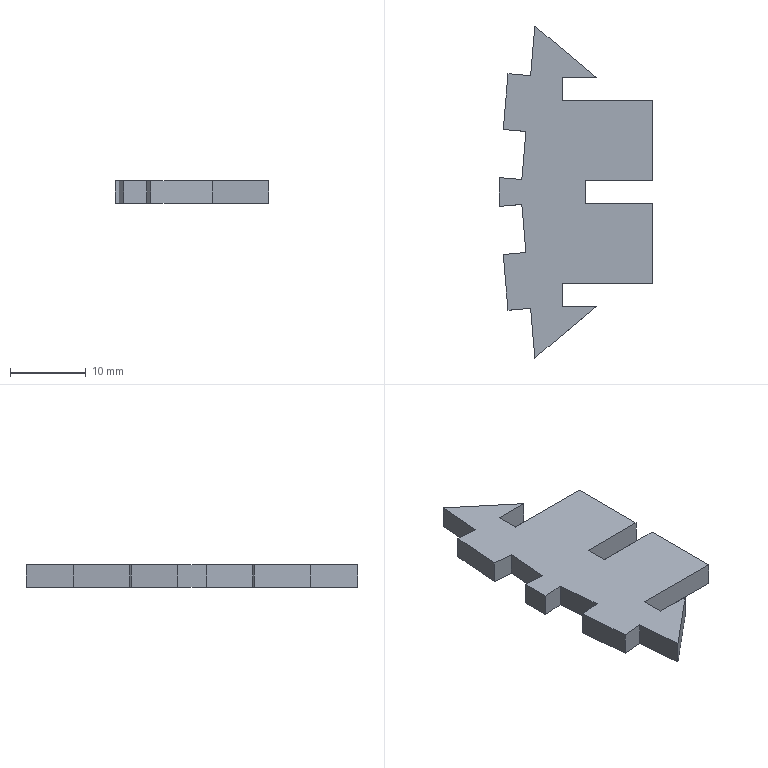Part | SolidWorks | features BaseBody 1 | 1 solid | 28 faces | box 20.269 x 43.799 x 3 mm | volume 1567 mm3 | plane 28
STEP:
#1=CARTESIAN_POINT('',(-11.851,-12.08,-1.5));
#2=VERTEX_POINT('',#1);
#3=CARTESIAN_POINT('',(0.1003,-12.082,-1.5));
#4=VERTEX_POINT('',#3);
#5=CARTESIAN_POINT('',(-0.002246,-12.082,-1.5));
#6=DIRECTION('',(1.,-0.0001859,0.));
#7=VECTOR('',#6,1000.);
#8=LINE('',#5,#7);
#9=EDGE_CURVE('',#2,#4,#8,.T.);
#10=ORIENTED_EDGE('',*,*,#9,.F.);
#11=CARTESIAN_POINT('',(-11.851,-15.077,-1.5));
#12=VERTEX_POINT('',#11);
#13=CARTESIAN_POINT('',(-11.851,0.,-1.5));
#14=DIRECTION('',(0.,1.,0.));
#15=VECTOR('',#14,1000.);
#16=LINE('',#13,#15);
#17=EDGE_CURVE('',#12,#2,#16,.T.);
#18=ORIENTED_EDGE('',*,*,#17,.F.);
#19=CARTESIAN_POINT('',(-7.293,-15.074,-1.5));
#20=VERTEX_POINT('',#19);
#21=CARTESIAN_POINT('',(0.009187,-15.07,-1.5));
#22=DIRECTION('',(-1.,-0.0006096,0.));
#23=VECTOR('',#22,1000.);
#24=LINE('',#21,#23);
#25=EDGE_CURVE('',#20,#12,#24,.T.);
#26=ORIENTED_EDGE('',*,*,#25,.F.);
#27=CARTESIAN_POINT('',(-15.47,-21.897,-1.5));
#28=VERTEX_POINT('',#27);
#29=CARTESIAN_POINT('',(4.421,-5.299,-1.5));
#30=DIRECTION('',(0.7678,0.6407,0.));
#31=VECTOR('',#30,1000.);
#32=LINE('',#29,#31);
#33=EDGE_CURVE('',#28,#20,#32,.T.);
#34=ORIENTED_EDGE('',*,*,#33,.F.);
#35=CARTESIAN_POINT('',(-16.025,-15.349,-1.5));
#36=VERTEX_POINT('',#35);
#37=CARTESIAN_POINT('',(-17.203,-1.458,-1.5));
#38=DIRECTION('',(0.08445,-0.9964,0.));
#39=VECTOR('',#38,1000.);
#40=LINE('',#37,#39);
#41=EDGE_CURVE('',#36,#28,#40,.T.);
#42=ORIENTED_EDGE('',*,*,#41,.F.);
#43=CARTESIAN_POINT('',(-19.01,-15.602,-1.5));
#44=VERTEX_POINT('',#43);
#45=CARTESIAN_POINT('',(1.175,-13.895,-1.5));
#46=DIRECTION('',(0.9964,0.08424,0.));
#47=VECTOR('',#46,1000.);
#48=LINE('',#45,#47);
#49=EDGE_CURVE('',#44,#36,#48,.T.);
#50=ORIENTED_EDGE('',*,*,#49,.F.);
#51=CARTESIAN_POINT('',(-19.632,-8.242,-1.5));
#52=VERTEX_POINT('',#51);
#53=CARTESIAN_POINT('',(-20.184,-1.706,-1.5));
#54=DIRECTION('',(0.08424,-0.9964,0.));
#55=VECTOR('',#54,1000.);
#56=LINE('',#53,#55);
#57=EDGE_CURVE('',#52,#44,#56,.T.);
#58=ORIENTED_EDGE('',*,*,#57,.F.);
#59=CARTESIAN_POINT('',(-16.646,-7.989,-1.5));
#60=VERTEX_POINT('',#59);
#61=CARTESIAN_POINT('',(0.5525,-6.535,-1.5));
#62=DIRECTION('',(-0.9964,-0.08424,0.));
#63=VECTOR('',#62,1000.);
#64=LINE('',#61,#63);
#65=EDGE_CURVE('',#60,#52,#64,.T.);
#66=ORIENTED_EDGE('',*,*,#65,.F.);
#67=CARTESIAN_POINT('',(-17.182,-1.643,-1.5));
#68=VERTEX_POINT('',#67);
#69=CARTESIAN_POINT('',(-17.198,-1.453,-1.5));
#70=DIRECTION('',(0.08416,-0.9965,0.));
#71=VECTOR('',#70,1000.);
#72=LINE('',#69,#71);
#73=EDGE_CURVE('',#68,#60,#72,.T.);
#74=ORIENTED_EDGE('',*,*,#73,.F.);
#75=CARTESIAN_POINT('',(-20.169,-1.897,-1.5));
#76=VERTEX_POINT('',#75);
#77=CARTESIAN_POINT('',(0.01566,-0.1847,-1.5));
#78=DIRECTION('',(0.9964,0.08451,0.));
#79=VECTOR('',#78,1000.);
#80=LINE('',#77,#79);
#81=EDGE_CURVE('',#76,#68,#80,.T.);
#82=ORIENTED_EDGE('',*,*,#81,.F.);
#83=CARTESIAN_POINT('',(-20.169,1.901,-1.5));
#84=VERTEX_POINT('',#83);
#85=CARTESIAN_POINT('',(-20.169,0.,-1.5));
#86=DIRECTION('',(0.,-1.,0.));
#87=VECTOR('',#86,1000.);
#88=LINE('',#85,#87);
#89=EDGE_CURVE('',#84,#76,#88,.T.);
#90=ORIENTED_EDGE('',*,*,#89,.F.);
#91=CARTESIAN_POINT('',(-17.182,1.648,-1.5));
#92=VERTEX_POINT('',#91);
#93=CARTESIAN_POINT('',(0.01606,0.1893,-1.5));
#94=DIRECTION('',(-0.9964,0.08451,0.));
#95=VECTOR('',#94,1000.);
#96=LINE('',#93,#95);
#97=EDGE_CURVE('',#92,#84,#96,.T.);
#98=ORIENTED_EDGE('',*,*,#97,.F.);
#99=CARTESIAN_POINT('',(-16.646,7.994,-1.5));
#100=VERTEX_POINT('',#99);
#101=CARTESIAN_POINT('',(-17.199,1.453,-1.5));
#102=DIRECTION('',(-0.08416,-0.9965,0.));
#103=VECTOR('',#102,1000.);
#104=LINE('',#101,#103);
#105=EDGE_CURVE('',#100,#92,#104,.T.);
#106=ORIENTED_EDGE('',*,*,#105,.F.);
#107=CARTESIAN_POINT('',(-19.632,8.246,-1.5));
#108=VERTEX_POINT('',#107);
#109=CARTESIAN_POINT('',(0.5529,6.54,-1.5));
#110=DIRECTION('',(0.9964,-0.08424,0.));
#111=VECTOR('',#110,1000.);
#112=LINE('',#109,#111);
#113=EDGE_CURVE('',#108,#100,#112,.T.);
#114=ORIENTED_EDGE('',*,*,#113,.F.);
#115=CARTESIAN_POINT('',(-19.01,15.606,-1.5));
#116=VERTEX_POINT('',#115);
#117=CARTESIAN_POINT('',(-20.185,1.706,-1.5));
#118=DIRECTION('',(-0.08424,-0.9964,0.));
#119=VECTOR('',#118,1000.);
#120=LINE('',#117,#119);
#121=EDGE_CURVE('',#116,#108,#120,.T.);
#122=ORIENTED_EDGE('',*,*,#121,.F.);
#123=CARTESIAN_POINT('',(-16.025,15.354,-1.5));
#124=VERTEX_POINT('',#123);
#125=CARTESIAN_POINT('',(1.175,13.9,-1.5));
#126=DIRECTION('',(-0.9964,0.08424,0.));
#127=VECTOR('',#126,1000.);
#128=LINE('',#125,#127);
#129=EDGE_CURVE('',#124,#116,#128,.T.);
#130=ORIENTED_EDGE('',*,*,#129,.F.);
#131=CARTESIAN_POINT('',(-15.47,21.902,-1.5));
#132=VERTEX_POINT('',#131);
#133=CARTESIAN_POINT('',(-17.203,1.458,-1.5));
#134=DIRECTION('',(-0.08445,-0.9964,0.));
#135=VECTOR('',#134,1000.);
#136=LINE('',#133,#135);
#137=EDGE_CURVE('',#132,#124,#136,.T.);
#138=ORIENTED_EDGE('',*,*,#137,.F.);
#139=CARTESIAN_POINT('',(-7.293,15.079,-1.5));
#140=VERTEX_POINT('',#139);
#141=CARTESIAN_POINT('',(4.424,5.301,-1.5));
#142=DIRECTION('',(-0.7678,0.6407,0.));
#143=VECTOR('',#142,1000.);
#144=LINE('',#141,#143);
#145=EDGE_CURVE('',#140,#132,#144,.T.);
#146=ORIENTED_EDGE('',*,*,#145,.F.);
#147=CARTESIAN_POINT('',(-11.851,15.082,-1.5));
#148=VERTEX_POINT('',#147);
#149=CARTESIAN_POINT('',(0.00919,15.074,-1.5));
#150=DIRECTION('',(1.,-0.0006096,0.));
#151=VECTOR('',#150,1000.);
#152=LINE('',#149,#151);
#153=EDGE_CURVE('',#148,#140,#152,.T.);
#154=ORIENTED_EDGE('',*,*,#153,.F.);
#155=CARTESIAN_POINT('',(-11.851,12.084,-1.5));
#156=VERTEX_POINT('',#155);
#157=CARTESIAN_POINT('',(-11.851,0.,-1.5));
#158=DIRECTION('',(0.,1.,0.));
#159=VECTOR('',#158,1000.);
#160=LINE('',#157,#159);
#161=EDGE_CURVE('',#156,#148,#160,.T.);
#162=ORIENTED_EDGE('',*,*,#161,.F.);
#163=CARTESIAN_POINT('',(0.1003,12.086,-1.5));
#164=VERTEX_POINT('',#163);
#165=CARTESIAN_POINT('',(-0.002247,12.086,-1.5));
#166=DIRECTION('',(-1.,-0.0001859,0.));
#167=VECTOR('',#166,1000.);
#168=LINE('',#165,#167);
#169=EDGE_CURVE('',#164,#156,#168,.T.);
#170=ORIENTED_EDGE('',*,*,#169,.F.);
#171=CARTESIAN_POINT('',(0.1003,1.498,-1.5));
#172=VERTEX_POINT('',#171);
#173=CARTESIAN_POINT('',(0.1003,0.,-1.5));
#174=DIRECTION('',(0.,1.,0.));
#175=VECTOR('',#174,1000.);
#176=LINE('',#173,#175);
#177=EDGE_CURVE('',#172,#164,#176,.T.);
#178=ORIENTED_EDGE('',*,*,#177,.F.);
#179=CARTESIAN_POINT('',(-8.819,1.498,-1.5));
#180=VERTEX_POINT('',#179);
#181=CARTESIAN_POINT('',(0.,1.498,-1.5));
#182=DIRECTION('',(1.,0.,0.));
#183=VECTOR('',#182,1000.);
#184=LINE('',#181,#183);
#185=EDGE_CURVE('',#180,#172,#184,.T.);
#186=ORIENTED_EDGE('',*,*,#185,.F.);
#187=CARTESIAN_POINT('',(-8.819,-1.498,-1.5));
#188=VERTEX_POINT('',#187);
#189=CARTESIAN_POINT('',(-8.819,0.,-1.5));
#190=DIRECTION('',(0.,1.,0.));
#191=VECTOR('',#190,1000.);
#192=LINE('',#189,#191);
#193=EDGE_CURVE('',#188,#180,#192,.T.);
#194=ORIENTED_EDGE('',*,*,#193,.F.);
#195=CARTESIAN_POINT('',(0.1003,-1.498,-1.5));
#196=VERTEX_POINT('',#195);
#197=CARTESIAN_POINT('',(0.,-1.498,-1.5));
#198=DIRECTION('',(-1.,0.,0.));
#199=VECTOR('',#198,1000.);
#200=LINE('',#197,#199);
#201=EDGE_CURVE('',#196,#188,#200,.T.);
#202=ORIENTED_EDGE('',*,*,#201,.F.);
#203=CARTESIAN_POINT('',(0.1003,0.,-1.5));
#204=DIRECTION('',(0.,1.,0.));
#205=VECTOR('',#204,1000.);
#206=LINE('',#203,#205);
#207=EDGE_CURVE('',#4,#196,#206,.T.);
#208=ORIENTED_EDGE('',*,*,#207,.F.);
#209=EDGE_LOOP('',(#10,#18,#26,#34,#42,#50,#58,#66,#74,#82,#90,#98,#106,#114,#122,#130,#138,#146,#154,#162,#170,#178,#186,#194,#202,#208));
#210=FACE_OUTER_BOUND('',#209,.T.);
#211=CARTESIAN_POINT('',(0.,0.,-1.5));
#212=DIRECTION('',(0.,0.,1.));
#213=DIRECTION('',(1.,0.,0.));
#214=AXIS2_PLACEMENT_3D('',#211,#212,#213);
#215=PLANE('',#214);
#216=ADVANCED_FACE('',(#210),#215,.F.);
#217=CARTESIAN_POINT('',(-11.851,-12.08,1.5));
#218=VERTEX_POINT('',#217);
#219=CARTESIAN_POINT('',(0.1003,-12.082,1.5));
#220=VERTEX_POINT('',#219);
#221=CARTESIAN_POINT('',(-0.002246,-12.082,1.5));
#222=DIRECTION('',(1.,-0.0001859,0.));
#223=VECTOR('',#222,1000.);
#224=LINE('',#221,#223);
#225=EDGE_CURVE('',#218,#220,#224,.T.);
#226=ORIENTED_EDGE('',*,*,#225,.T.);
#227=CARTESIAN_POINT('',(0.1003,-1.498,1.5));
#228=VERTEX_POINT('',#227);
#229=CARTESIAN_POINT('',(0.1003,0.,1.5));
#230=DIRECTION('',(0.,1.,0.));
#231=VECTOR('',#230,1000.);
#232=LINE('',#229,#231);
#233=EDGE_CURVE('',#220,#228,#232,.T.);
#234=ORIENTED_EDGE('',*,*,#233,.T.);
#235=CARTESIAN_POINT('',(-8.819,-1.498,1.5));
#236=VERTEX_POINT('',#235);
#237=CARTESIAN_POINT('',(0.,-1.498,1.5));
#238=DIRECTION('',(-1.,0.,0.));
#239=VECTOR('',#238,1000.);
#240=LINE('',#237,#239);
#241=EDGE_CURVE('',#228,#236,#240,.T.);
#242=ORIENTED_EDGE('',*,*,#241,.T.);
#243=CARTESIAN_POINT('',(-8.819,1.498,1.5));
#244=VERTEX_POINT('',#243);
#245=CARTESIAN_POINT('',(-8.819,0.,1.5));
#246=DIRECTION('',(0.,1.,0.));
#247=VECTOR('',#246,1000.);
#248=LINE('',#245,#247);
#249=EDGE_CURVE('',#236,#244,#248,.T.);
#250=ORIENTED_EDGE('',*,*,#249,.T.);
#251=CARTESIAN_POINT('',(0.1003,1.498,1.5));
#252=VERTEX_POINT('',#251);
#253=CARTESIAN_POINT('',(0.,1.498,1.5));
#254=DIRECTION('',(1.,0.,0.));
#255=VECTOR('',#254,1000.);
#256=LINE('',#253,#255);
#257=EDGE_CURVE('',#244,#252,#256,.T.);
#258=ORIENTED_EDGE('',*,*,#257,.T.);
#259=CARTESIAN_POINT('',(0.1003,12.086,1.5));
#260=VERTEX_POINT('',#259);
#261=CARTESIAN_POINT('',(0.1003,0.,1.5));
#262=DIRECTION('',(0.,1.,0.));
#263=VECTOR('',#262,1000.);
#264=LINE('',#261,#263);
#265=EDGE_CURVE('',#252,#260,#264,.T.);
#266=ORIENTED_EDGE('',*,*,#265,.T.);
#267=CARTESIAN_POINT('',(-11.851,12.084,1.5));
#268=VERTEX_POINT('',#267);
#269=CARTESIAN_POINT('',(-0.002247,12.086,1.5));
#270=DIRECTION('',(-1.,-0.0001859,0.));
#271=VECTOR('',#270,1000.);
#272=LINE('',#269,#271);
#273=EDGE_CURVE('',#260,#268,#272,.T.);
#274=ORIENTED_EDGE('',*,*,#273,.T.);
#275=CARTESIAN_POINT('',(-11.851,15.082,1.5));
#276=VERTEX_POINT('',#275);
#277=CARTESIAN_POINT('',(-11.851,0.,1.5));
#278=DIRECTION('',(0.,1.,0.));
#279=VECTOR('',#278,1000.);
#280=LINE('',#277,#279);
#281=EDGE_CURVE('',#268,#276,#280,.T.);
#282=ORIENTED_EDGE('',*,*,#281,.T.);
#283=CARTESIAN_POINT('',(-7.293,15.079,1.5));
#284=VERTEX_POINT('',#283);
#285=CARTESIAN_POINT('',(0.00919,15.074,1.5));
#286=DIRECTION('',(1.,-0.0006096,0.));
#287=VECTOR('',#286,1000.);
#288=LINE('',#285,#287);
#289=EDGE_CURVE('',#276,#284,#288,.T.);
#290=ORIENTED_EDGE('',*,*,#289,.T.);
#291=CARTESIAN_POINT('',(-15.47,21.902,1.5));
#292=VERTEX_POINT('',#291);
#293=CARTESIAN_POINT('',(4.424,5.301,1.5));
#294=DIRECTION('',(-0.7678,0.6407,0.));
#295=VECTOR('',#294,1000.);
#296=LINE('',#293,#295);
#297=EDGE_CURVE('',#284,#292,#296,.T.);
#298=ORIENTED_EDGE('',*,*,#297,.T.);
#299=CARTESIAN_POINT('',(-16.025,15.354,1.5));
#300=VERTEX_POINT('',#299);
#301=CARTESIAN_POINT('',(-17.203,1.458,1.5));
#302=DIRECTION('',(-0.08445,-0.9964,0.));
#303=VECTOR('',#302,1000.);
#304=LINE('',#301,#303);
#305=EDGE_CURVE('',#292,#300,#304,.T.);
#306=ORIENTED_EDGE('',*,*,#305,.T.);
#307=CARTESIAN_POINT('',(-19.01,15.606,1.5));
#308=VERTEX_POINT('',#307);
#309=CARTESIAN_POINT('',(1.175,13.9,1.5));
#310=DIRECTION('',(-0.9964,0.08424,0.));
#311=VECTOR('',#310,1000.);
#312=LINE('',#309,#311);
#313=EDGE_CURVE('',#300,#308,#312,.T.);
#314=ORIENTED_EDGE('',*,*,#313,.T.);
#315=CARTESIAN_POINT('',(-19.632,8.246,1.5));
#316=VERTEX_POINT('',#315);
#317=CARTESIAN_POINT('',(-20.185,1.706,1.5));
#318=DIRECTION('',(-0.08424,-0.9964,0.));
#319=VECTOR('',#318,1000.);
#320=LINE('',#317,#319);
#321=EDGE_CURVE('',#308,#316,#320,.T.);
#322=ORIENTED_EDGE('',*,*,#321,.T.);
#323=CARTESIAN_POINT('',(-16.646,7.994,1.5));
#324=VERTEX_POINT('',#323);
#325=CARTESIAN_POINT('',(0.5529,6.54,1.5));
#326=DIRECTION('',(0.9964,-0.08424,0.));
#327=VECTOR('',#326,1000.);
#328=LINE('',#325,#327);
#329=EDGE_CURVE('',#316,#324,#328,.T.);
#330=ORIENTED_EDGE('',*,*,#329,.T.);
#331=CARTESIAN_POINT('',(-17.182,1.648,1.5));
#332=VERTEX_POINT('',#331);
#333=CARTESIAN_POINT('',(-17.199,1.453,1.5));
#334=DIRECTION('',(-0.08416,-0.9965,0.));
#335=VECTOR('',#334,1000.);
#336=LINE('',#333,#335);
#337=EDGE_CURVE('',#324,#332,#336,.T.);
#338=ORIENTED_EDGE('',*,*,#337,.T.);
#339=CARTESIAN_POINT('',(-20.169,1.901,1.5));
#340=VERTEX_POINT('',#339);
#341=CARTESIAN_POINT('',(0.01606,0.1893,1.5));
#342=DIRECTION('',(-0.9964,0.08451,0.));
#343=VECTOR('',#342,1000.);
#344=LINE('',#341,#343);
#345=EDGE_CURVE('',#332,#340,#344,.T.);
#346=ORIENTED_EDGE('',*,*,#345,.T.);
#347=CARTESIAN_POINT('',(-20.169,-1.897,1.5));
#348=VERTEX_POINT('',#347);
#349=CARTESIAN_POINT('',(-20.169,0.,1.5));
#350=DIRECTION('',(0.,-1.,0.));
#351=VECTOR('',#350,1000.);
#352=LINE('',#349,#351);
#353=EDGE_CURVE('',#340,#348,#352,.T.);
#354=ORIENTED_EDGE('',*,*,#353,.T.);
#355=CARTESIAN_POINT('',(-17.182,-1.643,1.5));
#356=VERTEX_POINT('',#355);
#357=CARTESIAN_POINT('',(0.01566,-0.1847,1.5));
#358=DIRECTION('',(0.9964,0.08451,0.));
#359=VECTOR('',#358,1000.);
#360=LINE('',#357,#359);
#361=EDGE_CURVE('',#348,#356,#360,.T.);
#362=ORIENTED_EDGE('',*,*,#361,.T.);
#363=CARTESIAN_POINT('',(-16.646,-7.989,1.5));
#364=VERTEX_POINT('',#363);
#365=CARTESIAN_POINT('',(-17.198,-1.453,1.5));
#366=DIRECTION('',(0.08416,-0.9965,0.));
#367=VECTOR('',#366,1000.);
#368=LINE('',#365,#367);
#369=EDGE_CURVE('',#356,#364,#368,.T.);
#370=ORIENTED_EDGE('',*,*,#369,.T.);
#371=CARTESIAN_POINT('',(-19.632,-8.242,1.5));
#372=VERTEX_POINT('',#371);
#373=CARTESIAN_POINT('',(0.5525,-6.535,1.5));
#374=DIRECTION('',(-0.9964,-0.08424,0.));
#375=VECTOR('',#374,1000.);
#376=LINE('',#373,#375);
#377=EDGE_CURVE('',#364,#372,#376,.T.);
#378=ORIENTED_EDGE('',*,*,#377,.T.);
#379=CARTESIAN_POINT('',(-19.01,-15.602,1.5));
#380=VERTEX_POINT('',#379);
#381=CARTESIAN_POINT('',(-20.184,-1.706,1.5));
#382=DIRECTION('',(0.08424,-0.9964,0.));
#383=VECTOR('',#382,1000.);
#384=LINE('',#381,#383);
#385=EDGE_CURVE('',#372,#380,#384,.T.);
#386=ORIENTED_EDGE('',*,*,#385,.T.);
#387=CARTESIAN_POINT('',(-16.025,-15.349,1.5));
#388=VERTEX_POINT('',#387);
#389=CARTESIAN_POINT('',(1.175,-13.895,1.5));
#390=DIRECTION('',(0.9964,0.08424,0.));
#391=VECTOR('',#390,1000.);
#392=LINE('',#389,#391);
#393=EDGE_CURVE('',#380,#388,#392,.T.);
#394=ORIENTED_EDGE('',*,*,#393,.T.);
#395=CARTESIAN_POINT('',(-15.47,-21.897,1.5));
#396=VERTEX_POINT('',#395);
#397=CARTESIAN_POINT('',(-17.203,-1.458,1.5));
#398=DIRECTION('',(0.08445,-0.9964,0.));
#399=VECTOR('',#398,1000.);
#400=LINE('',#397,#399);
#401=EDGE_CURVE('',#388,#396,#400,.T.);
#402=ORIENTED_EDGE('',*,*,#401,.T.);
#403=CARTESIAN_POINT('',(-7.293,-15.074,1.5));
#404=VERTEX_POINT('',#403);
#405=CARTESIAN_POINT('',(4.421,-5.299,1.5));
#406=DIRECTION('',(0.7678,0.6407,0.));
#407=VECTOR('',#406,1000.);
#408=LINE('',#405,#407);
#409=EDGE_CURVE('',#396,#404,#408,.T.);
#410=ORIENTED_EDGE('',*,*,#409,.T.);
#411=CARTESIAN_POINT('',(-11.851,-15.077,1.5));
#412=VERTEX_POINT('',#411);
#413=CARTESIAN_POINT('',(0.009187,-15.07,1.5));
#414=DIRECTION('',(-1.,-0.0006096,0.));
#415=VECTOR('',#414,1000.);
#416=LINE('',#413,#415);
#417=EDGE_CURVE('',#404,#412,#416,.T.);
#418=ORIENTED_EDGE('',*,*,#417,.T.);
#419=CARTESIAN_POINT('',(-11.851,0.,1.5));
#420=DIRECTION('',(0.,1.,0.));
#421=VECTOR('',#420,1000.);
#422=LINE('',#419,#421);
#423=EDGE_CURVE('',#412,#218,#422,.T.);
#424=ORIENTED_EDGE('',*,*,#423,.T.);
#425=EDGE_LOOP('',(#226,#234,#242,#250,#258,#266,#274,#282,#290,#298,#306,#314,#322,#330,#338,#346,#354,#362,#370,#378,#386,#394,#402,#410,#418,#424));
#426=FACE_OUTER_BOUND('',#425,.T.);
#427=CARTESIAN_POINT('',(0.,0.,1.5));
#428=DIRECTION('',(0.,0.,1.));
#429=DIRECTION('',(1.,0.,0.));
#430=AXIS2_PLACEMENT_3D('',#427,#428,#429);
#431=PLANE('',#430);
#432=ADVANCED_FACE('',(#426),#431,.T.);
#433=ORIENTED_EDGE('',*,*,#17,.T.);
#434=CARTESIAN_POINT('',(-11.851,-12.08,1.5));
#435=DIRECTION('',(0.,0.,-1.));
#436=VECTOR('',#435,1000.);
#437=LINE('',#434,#436);
#438=EDGE_CURVE('',#218,#2,#437,.T.);
#439=ORIENTED_EDGE('',*,*,#438,.F.);
#440=ORIENTED_EDGE('',*,*,#423,.F.);
#441=CARTESIAN_POINT('',(-11.851,-15.077,1.5));
#442=DIRECTION('',(0.,0.,-1.));
#443=VECTOR('',#442,1000.);
#444=LINE('',#441,#443);
#445=EDGE_CURVE('',#412,#12,#444,.T.);
#446=ORIENTED_EDGE('',*,*,#445,.T.);
#447=EDGE_LOOP('',(#433,#439,#440,#446));
#448=FACE_OUTER_BOUND('',#447,.T.);
#449=CARTESIAN_POINT('',(-11.851,0.,1.5));
#450=DIRECTION('',(-1.,0.,0.));
#451=DIRECTION('',(0.,0.,1.));
#452=AXIS2_PLACEMENT_3D('',#449,#450,#451);
#453=PLANE('',#452);
#454=ADVANCED_FACE('',(#448),#453,.F.);
#455=ORIENTED_EDGE('',*,*,#25,.T.);
#456=ORIENTED_EDGE('',*,*,#445,.F.);
#457=ORIENTED_EDGE('',*,*,#417,.F.);
#458=CARTESIAN_POINT('',(-7.293,-15.074,1.5));
#459=DIRECTION('',(0.,0.,-1.));
#460=VECTOR('',#459,1000.);
#461=LINE('',#458,#460);
#462=EDGE_CURVE('',#404,#20,#461,.T.);
#463=ORIENTED_EDGE('',*,*,#462,.T.);
#464=EDGE_LOOP('',(#455,#456,#457,#463));
#465=FACE_OUTER_BOUND('',#464,.T.);
#466=CARTESIAN_POINT('',(0.009187,-15.07,1.5));
#467=DIRECTION('',(0.0006096,-1.,0.));
#468=DIRECTION('',(0.,0.,-1.));
#469=AXIS2_PLACEMENT_3D('',#466,#467,#468);
#470=PLANE('',#469);
#471=ADVANCED_FACE('',(#465),#470,.F.);
#472=ORIENTED_EDGE('',*,*,#33,.T.);
#473=ORIENTED_EDGE('',*,*,#462,.F.);
#474=ORIENTED_EDGE('',*,*,#409,.F.);
#475=CARTESIAN_POINT('',(-15.47,-21.897,1.5));
#476=DIRECTION('',(0.,0.,-1.));
#477=VECTOR('',#476,1000.);
#478=LINE('',#475,#477);
#479=EDGE_CURVE('',#396,#28,#478,.T.);
#480=ORIENTED_EDGE('',*,*,#479,.T.);
#481=EDGE_LOOP('',(#472,#473,#474,#480));
#482=FACE_OUTER_BOUND('',#481,.T.);
#483=CARTESIAN_POINT('',(4.421,-5.299,1.5));
#484=DIRECTION('',(-0.6407,0.7678,0.));
#485=DIRECTION('',(0.,0.,1.));
#486=AXIS2_PLACEMENT_3D('',#483,#484,#485);
#487=PLANE('',#486);
#488=ADVANCED_FACE('',(#482),#487,.F.);
#489=ORIENTED_EDGE('',*,*,#41,.T.);
#490=ORIENTED_EDGE('',*,*,#479,.F.);
#491=ORIENTED_EDGE('',*,*,#401,.F.);
#492=CARTESIAN_POINT('',(-16.025,-15.349,1.5));
#493=DIRECTION('',(0.,0.,-1.));
#494=VECTOR('',#493,1000.);
#495=LINE('',#492,#494);
#496=EDGE_CURVE('',#388,#36,#495,.T.);
#497=ORIENTED_EDGE('',*,*,#496,.T.);
#498=EDGE_LOOP('',(#489,#490,#491,#497));
#499=FACE_OUTER_BOUND('',#498,.T.);
#500=CARTESIAN_POINT('',(-17.203,-1.458,1.5));
#501=DIRECTION('',(0.9964,0.08445,0.));
#502=DIRECTION('',(0.,0.,-1.));
#503=AXIS2_PLACEMENT_3D('',#500,#501,#502);
#504=PLANE('',#503);
#505=ADVANCED_FACE('',(#499),#504,.F.);
#506=ORIENTED_EDGE('',*,*,#49,.T.);
#507=ORIENTED_EDGE('',*,*,#496,.F.);
#508=ORIENTED_EDGE('',*,*,#393,.F.);
#509=CARTESIAN_POINT('',(-19.01,-15.602,1.5));
#510=DIRECTION('',(0.,0.,-1.));
#511=VECTOR('',#510,1000.);
#512=LINE('',#509,#511);
#513=EDGE_CURVE('',#380,#44,#512,.T.);
#514=ORIENTED_EDGE('',*,*,#513,.T.);
#515=EDGE_LOOP('',(#506,#507,#508,#514));
#516=FACE_OUTER_BOUND('',#515,.T.);
#517=CARTESIAN_POINT('',(1.175,-13.895,1.5));
#518=DIRECTION('',(-0.08424,0.9964,0.));
#519=DIRECTION('',(0.,0.,1.));
#520=AXIS2_PLACEMENT_3D('',#517,#518,#519);
#521=PLANE('',#520);
#522=ADVANCED_FACE('',(#516),#521,.F.);
#523=ORIENTED_EDGE('',*,*,#57,.T.);
#524=ORIENTED_EDGE('',*,*,#513,.F.);
#525=ORIENTED_EDGE('',*,*,#385,.F.);
#526=CARTESIAN_POINT('',(-19.632,-8.242,1.5));
#527=DIRECTION('',(0.,0.,-1.));
#528=VECTOR('',#527,1000.);
#529=LINE('',#526,#528);
#530=EDGE_CURVE('',#372,#52,#529,.T.);
#531=ORIENTED_EDGE('',*,*,#530,.T.);
#532=EDGE_LOOP('',(#523,#524,#525,#531));
#533=FACE_OUTER_BOUND('',#532,.T.);
#534=CARTESIAN_POINT('',(-20.184,-1.706,1.5));
#535=DIRECTION('',(0.9964,0.08424,0.));
#536=DIRECTION('',(0.,0.,-1.));
#537=AXIS2_PLACEMENT_3D('',#534,#535,#536);
#538=PLANE('',#537);
#539=ADVANCED_FACE('',(#533),#538,.F.);
#540=ORIENTED_EDGE('',*,*,#65,.T.);
#541=ORIENTED_EDGE('',*,*,#530,.F.);
#542=ORIENTED_EDGE('',*,*,#377,.F.);
#543=CARTESIAN_POINT('',(-16.646,-7.989,1.5));
#544=DIRECTION('',(0.,0.,-1.));
#545=VECTOR('',#544,1000.);
#546=LINE('',#543,#545);
#547=EDGE_CURVE('',#364,#60,#546,.T.);
#548=ORIENTED_EDGE('',*,*,#547,.T.);
#549=EDGE_LOOP('',(#540,#541,#542,#548));
#550=FACE_OUTER_BOUND('',#549,.T.);
#551=CARTESIAN_POINT('',(0.5525,-6.535,1.5));
#552=DIRECTION('',(0.08424,-0.9964,0.));
#553=DIRECTION('',(0.,0.,-1.));
#554=AXIS2_PLACEMENT_3D('',#551,#552,#553);
#555=PLANE('',#554);
#556=ADVANCED_FACE('',(#550),#555,.F.);
#557=ORIENTED_EDGE('',*,*,#73,.T.);
#558=ORIENTED_EDGE('',*,*,#547,.F.);
#559=ORIENTED_EDGE('',*,*,#369,.F.);
#560=CARTESIAN_POINT('',(-17.182,-1.643,1.5));
#561=DIRECTION('',(0.,0.,-1.));
#562=VECTOR('',#561,1000.);
#563=LINE('',#560,#562);
#564=EDGE_CURVE('',#356,#68,#563,.T.);
#565=ORIENTED_EDGE('',*,*,#564,.T.);
#566=EDGE_LOOP('',(#557,#558,#559,#565));
#567=FACE_OUTER_BOUND('',#566,.T.);
#568=CARTESIAN_POINT('',(-17.198,-1.453,1.5));
#569=DIRECTION('',(0.9965,0.08416,0.));
#570=DIRECTION('',(0.,0.,-1.));
#571=AXIS2_PLACEMENT_3D('',#568,#569,#570);
#572=PLANE('',#571);
#573=ADVANCED_FACE('',(#567),#572,.F.);
#574=ORIENTED_EDGE('',*,*,#81,.T.);
#575=ORIENTED_EDGE('',*,*,#564,.F.);
#576=ORIENTED_EDGE('',*,*,#361,.F.);
#577=CARTESIAN_POINT('',(-20.169,-1.897,1.5));
#578=DIRECTION('',(0.,0.,-1.));
#579=VECTOR('',#578,1000.);
#580=LINE('',#577,#579);
#581=EDGE_CURVE('',#348,#76,#580,.T.);
#582=ORIENTED_EDGE('',*,*,#581,.T.);
#583=EDGE_LOOP('',(#574,#575,#576,#582));
#584=FACE_OUTER_BOUND('',#583,.T.);
#585=CARTESIAN_POINT('',(0.01566,-0.1847,1.5));
#586=DIRECTION('',(-0.08451,0.9964,0.));
#587=DIRECTION('',(0.,0.,1.));
#588=AXIS2_PLACEMENT_3D('',#585,#586,#587);
#589=PLANE('',#588);
#590=ADVANCED_FACE('',(#584),#589,.F.);
#591=ORIENTED_EDGE('',*,*,#89,.T.);
#592=ORIENTED_EDGE('',*,*,#581,.F.);
#593=ORIENTED_EDGE('',*,*,#353,.F.);
#594=CARTESIAN_POINT('',(-20.169,1.901,1.5));
#595=DIRECTION('',(0.,0.,-1.));
#596=VECTOR('',#595,1000.);
#597=LINE('',#594,#596);
#598=EDGE_CURVE('',#340,#84,#597,.T.);
#599=ORIENTED_EDGE('',*,*,#598,.T.);
#600=EDGE_LOOP('',(#591,#592,#593,#599));
#601=FACE_OUTER_BOUND('',#600,.T.);
#602=CARTESIAN_POINT('',(-20.169,0.,1.5));
#603=DIRECTION('',(1.,0.,0.));
#604=DIRECTION('',(0.,1.,0.));
#605=AXIS2_PLACEMENT_3D('',#602,#603,#604);
#606=PLANE('',#605);
#607=ADVANCED_FACE('',(#601),#606,.F.);
#608=ORIENTED_EDGE('',*,*,#97,.T.);
#609=ORIENTED_EDGE('',*,*,#598,.F.);
#610=ORIENTED_EDGE('',*,*,#345,.F.);
#611=CARTESIAN_POINT('',(-17.182,1.648,1.5));
#612=DIRECTION('',(0.,0.,-1.));
#613=VECTOR('',#612,1000.);
#614=LINE('',#611,#613);
#615=EDGE_CURVE('',#332,#92,#614,.T.);
#616=ORIENTED_EDGE('',*,*,#615,.T.);
#617=EDGE_LOOP('',(#608,#609,#610,#616));
#618=FACE_OUTER_BOUND('',#617,.T.);
#619=CARTESIAN_POINT('',(0.01606,0.1893,1.5));
#620=DIRECTION('',(-0.08451,-0.9964,0.));
#621=DIRECTION('',(-0.9964,0.08451,0.));
#622=AXIS2_PLACEMENT_3D('',#619,#620,#621);
#623=PLANE('',#622);
#624=ADVANCED_FACE('',(#618),#623,.F.);
#625=ORIENTED_EDGE('',*,*,#105,.T.);
#626=ORIENTED_EDGE('',*,*,#615,.F.);
#627=ORIENTED_EDGE('',*,*,#337,.F.);
#628=CARTESIAN_POINT('',(-16.646,7.994,1.5));
#629=DIRECTION('',(0.,0.,-1.));
#630=VECTOR('',#629,1000.);
#631=LINE('',#628,#630);
#632=EDGE_CURVE('',#324,#100,#631,.T.);
#633=ORIENTED_EDGE('',*,*,#632,.T.);
#634=EDGE_LOOP('',(#625,#626,#627,#633));
#635=FACE_OUTER_BOUND('',#634,.T.);
#636=CARTESIAN_POINT('',(-17.199,1.453,1.5));
#637=DIRECTION('',(0.9965,-0.08416,0.));
#638=DIRECTION('',(0.,0.,-1.));
#639=AXIS2_PLACEMENT_3D('',#636,#637,#638);
#640=PLANE('',#639);
#641=ADVANCED_FACE('',(#635),#640,.F.);
#642=ORIENTED_EDGE('',*,*,#113,.T.);
#643=ORIENTED_EDGE('',*,*,#632,.F.);
#644=ORIENTED_EDGE('',*,*,#329,.F.);
#645=CARTESIAN_POINT('',(-19.632,8.246,1.5));
#646=DIRECTION('',(0.,0.,-1.));
#647=VECTOR('',#646,1000.);
#648=LINE('',#645,#647);
#649=EDGE_CURVE('',#316,#108,#648,.T.);
#650=ORIENTED_EDGE('',*,*,#649,.T.);
#651=EDGE_LOOP('',(#642,#643,#644,#650));
#652=FACE_OUTER_BOUND('',#651,.T.);
#653=CARTESIAN_POINT('',(0.5529,6.54,1.5));
#654=DIRECTION('',(0.08424,0.9964,0.));
#655=DIRECTION('',(0.,0.,-1.));
#656=AXIS2_PLACEMENT_3D('',#653,#654,#655);
#657=PLANE('',#656);
#658=ADVANCED_FACE('',(#652),#657,.F.);
#659=ORIENTED_EDGE('',*,*,#121,.T.);
#660=ORIENTED_EDGE('',*,*,#649,.F.);
#661=ORIENTED_EDGE('',*,*,#321,.F.);
#662=CARTESIAN_POINT('',(-19.01,15.606,1.5));
#663=DIRECTION('',(0.,0.,-1.));
#664=VECTOR('',#663,1000.);
#665=LINE('',#662,#664);
#666=EDGE_CURVE('',#308,#116,#665,.T.);
#667=ORIENTED_EDGE('',*,*,#666,.T.);
#668=EDGE_LOOP('',(#659,#660,#661,#667));
#669=FACE_OUTER_BOUND('',#668,.T.);
#670=CARTESIAN_POINT('',(-20.185,1.706,1.5));
#671=DIRECTION('',(0.9964,-0.08424,0.));
#672=DIRECTION('',(0.,0.,-1.));
#673=AXIS2_PLACEMENT_3D('',#670,#671,#672);
#674=PLANE('',#673);
#675=ADVANCED_FACE('',(#669),#674,.F.);
#676=ORIENTED_EDGE('',*,*,#129,.T.);
#677=ORIENTED_EDGE('',*,*,#666,.F.);
#678=ORIENTED_EDGE('',*,*,#313,.F.);
#679=CARTESIAN_POINT('',(-16.025,15.354,1.5));
#680=DIRECTION('',(0.,0.,-1.));
#681=VECTOR('',#680,1000.);
#682=LINE('',#679,#681);
#683=EDGE_CURVE('',#300,#124,#682,.T.);
#684=ORIENTED_EDGE('',*,*,#683,.T.);
#685=EDGE_LOOP('',(#676,#677,#678,#684));
#686=FACE_OUTER_BOUND('',#685,.T.);
#687=CARTESIAN_POINT('',(1.175,13.9,1.5));
#688=DIRECTION('',(-0.08424,-0.9964,0.));
#689=DIRECTION('',(-0.9964,0.08424,0.));
#690=AXIS2_PLACEMENT_3D('',#687,#688,#689);
#691=PLANE('',#690);
#692=ADVANCED_FACE('',(#686),#691,.F.);
#693=ORIENTED_EDGE('',*,*,#137,.T.);
#694=ORIENTED_EDGE('',*,*,#683,.F.);
#695=ORIENTED_EDGE('',*,*,#305,.F.);
#696=CARTESIAN_POINT('',(-15.47,21.902,1.5));
#697=DIRECTION('',(0.,0.,-1.));
#698=VECTOR('',#697,1000.);
#699=LINE('',#696,#698);
#700=EDGE_CURVE('',#292,#132,#699,.T.);
#701=ORIENTED_EDGE('',*,*,#700,.T.);
#702=EDGE_LOOP('',(#693,#694,#695,#701));
#703=FACE_OUTER_BOUND('',#702,.T.);
#704=CARTESIAN_POINT('',(-17.203,1.458,1.5));
#705=DIRECTION('',(0.9964,-0.08445,0.));
#706=DIRECTION('',(0.,0.,-1.));
#707=AXIS2_PLACEMENT_3D('',#704,#705,#706);
#708=PLANE('',#707);
#709=ADVANCED_FACE('',(#703),#708,.F.);
#710=ORIENTED_EDGE('',*,*,#145,.T.);
#711=ORIENTED_EDGE('',*,*,#700,.F.);
#712=ORIENTED_EDGE('',*,*,#297,.F.);
#713=CARTESIAN_POINT('',(-7.293,15.079,1.5));
#714=DIRECTION('',(0.,0.,-1.));
#715=VECTOR('',#714,1000.);
#716=LINE('',#713,#715);
#717=EDGE_CURVE('',#284,#140,#716,.T.);
#718=ORIENTED_EDGE('',*,*,#717,.T.);
#719=EDGE_LOOP('',(#710,#711,#712,#718));
#720=FACE_OUTER_BOUND('',#719,.T.);
#721=CARTESIAN_POINT('',(4.424,5.301,1.5));
#722=DIRECTION('',(-0.6407,-0.7678,0.));
#723=DIRECTION('',(-0.7678,0.6407,0.));
#724=AXIS2_PLACEMENT_3D('',#721,#722,#723);
#725=PLANE('',#724);
#726=ADVANCED_FACE('',(#720),#725,.F.);
#727=ORIENTED_EDGE('',*,*,#153,.T.);
#728=ORIENTED_EDGE('',*,*,#717,.F.);
#729=ORIENTED_EDGE('',*,*,#289,.F.);
#730=CARTESIAN_POINT('',(-11.851,15.082,1.5));
#731=DIRECTION('',(0.,0.,-1.));
#732=VECTOR('',#731,1000.);
#733=LINE('',#730,#732);
#734=EDGE_CURVE('',#276,#148,#733,.T.);
#735=ORIENTED_EDGE('',*,*,#734,.T.);
#736=EDGE_LOOP('',(#727,#728,#729,#735));
#737=FACE_OUTER_BOUND('',#736,.T.);
#738=CARTESIAN_POINT('',(0.00919,15.074,1.5));
#739=DIRECTION('',(0.0006096,1.,0.));
#740=DIRECTION('',(0.,0.,-1.));
#741=AXIS2_PLACEMENT_3D('',#738,#739,#740);
#742=PLANE('',#741);
#743=ADVANCED_FACE('',(#737),#742,.F.);
#744=ORIENTED_EDGE('',*,*,#161,.T.);
#745=ORIENTED_EDGE('',*,*,#734,.F.);
#746=ORIENTED_EDGE('',*,*,#281,.F.);
#747=CARTESIAN_POINT('',(-11.851,12.084,1.5));
#748=DIRECTION('',(0.,0.,-1.));
#749=VECTOR('',#748,1000.);
#750=LINE('',#747,#749);
#751=EDGE_CURVE('',#268,#156,#750,.T.);
#752=ORIENTED_EDGE('',*,*,#751,.T.);
#753=EDGE_LOOP('',(#744,#745,#746,#752));
#754=FACE_OUTER_BOUND('',#753,.T.);
#755=CARTESIAN_POINT('',(-11.851,0.,1.5));
#756=DIRECTION('',(-1.,0.,0.));
#757=DIRECTION('',(0.,0.,1.));
#758=AXIS2_PLACEMENT_3D('',#755,#756,#757);
#759=PLANE('',#758);
#760=ADVANCED_FACE('',(#754),#759,.F.);
#761=ORIENTED_EDGE('',*,*,#169,.T.);
#762=ORIENTED_EDGE('',*,*,#751,.F.);
#763=ORIENTED_EDGE('',*,*,#273,.F.);
#764=CARTESIAN_POINT('',(0.1003,12.086,1.5));
#765=DIRECTION('',(0.,0.,-1.));
#766=VECTOR('',#765,1000.);
#767=LINE('',#764,#766);
#768=EDGE_CURVE('',#260,#164,#767,.T.);
#769=ORIENTED_EDGE('',*,*,#768,.T.);
#770=EDGE_LOOP('',(#761,#762,#763,#769));
#771=FACE_OUTER_BOUND('',#770,.T.);
#772=CARTESIAN_POINT('',(-0.002247,12.086,1.5));
#773=DIRECTION('',(0.0001859,-1.,0.));
#774=DIRECTION('',(0.,0.,-1.));
#775=AXIS2_PLACEMENT_3D('',#772,#773,#774);
#776=PLANE('',#775);
#777=ADVANCED_FACE('',(#771),#776,.F.);
#778=ORIENTED_EDGE('',*,*,#177,.T.);
#779=ORIENTED_EDGE('',*,*,#768,.F.);
#780=ORIENTED_EDGE('',*,*,#265,.F.);
#781=CARTESIAN_POINT('',(0.1003,1.498,1.5));
#782=DIRECTION('',(0.,0.,-1.));
#783=VECTOR('',#782,1000.);
#784=LINE('',#781,#783);
#785=EDGE_CURVE('',#252,#172,#784,.T.);
#786=ORIENTED_EDGE('',*,*,#785,.T.);
#787=EDGE_LOOP('',(#778,#779,#780,#786));
#788=FACE_OUTER_BOUND('',#787,.T.);
#789=CARTESIAN_POINT('',(0.1003,0.,1.5));
#790=DIRECTION('',(-1.,0.,0.));
#791=DIRECTION('',(0.,0.,1.));
#792=AXIS2_PLACEMENT_3D('',#789,#790,#791);
#793=PLANE('',#792);
#794=ADVANCED_FACE('',(#788),#793,.F.);
#795=ORIENTED_EDGE('',*,*,#185,.T.);
#796=ORIENTED_EDGE('',*,*,#785,.F.);
#797=ORIENTED_EDGE('',*,*,#257,.F.);
#798=CARTESIAN_POINT('',(-8.819,1.498,1.5));
#799=DIRECTION('',(0.,0.,-1.));
#800=VECTOR('',#799,1000.);
#801=LINE('',#798,#800);
#802=EDGE_CURVE('',#244,#180,#801,.T.);
#803=ORIENTED_EDGE('',*,*,#802,.T.);
#804=EDGE_LOOP('',(#795,#796,#797,#803));
#805=FACE_OUTER_BOUND('',#804,.T.);
#806=CARTESIAN_POINT('',(0.,1.498,1.5));
#807=DIRECTION('',(0.,1.,0.));
#808=DIRECTION('',(1.,0.,0.));
#809=AXIS2_PLACEMENT_3D('',#806,#807,#808);
#810=PLANE('',#809);
#811=ADVANCED_FACE('',(#805),#810,.F.);
#812=ORIENTED_EDGE('',*,*,#193,.T.);
#813=ORIENTED_EDGE('',*,*,#802,.F.);
#814=ORIENTED_EDGE('',*,*,#249,.F.);
#815=CARTESIAN_POINT('',(-8.819,-1.498,1.5));
#816=DIRECTION('',(0.,0.,-1.));
#817=VECTOR('',#816,1000.);
#818=LINE('',#815,#817);
#819=EDGE_CURVE('',#236,#188,#818,.T.);
#820=ORIENTED_EDGE('',*,*,#819,.T.);
#821=EDGE_LOOP('',(#812,#813,#814,#820));
#822=FACE_OUTER_BOUND('',#821,.T.);
#823=CARTESIAN_POINT('',(-8.819,0.,1.5));
#824=DIRECTION('',(-1.,0.,0.));
#825=DIRECTION('',(0.,0.,1.));
#826=AXIS2_PLACEMENT_3D('',#823,#824,#825);
#827=PLANE('',#826);
#828=ADVANCED_FACE('',(#822),#827,.F.);
#829=ORIENTED_EDGE('',*,*,#201,.T.);
#830=ORIENTED_EDGE('',*,*,#819,.F.);
#831=ORIENTED_EDGE('',*,*,#241,.F.);
#832=CARTESIAN_POINT('',(0.1003,-1.498,1.5));
#833=DIRECTION('',(0.,0.,-1.));
#834=VECTOR('',#833,1000.);
#835=LINE('',#832,#834);
#836=EDGE_CURVE('',#228,#196,#835,.T.);
#837=ORIENTED_EDGE('',*,*,#836,.T.);
#838=EDGE_LOOP('',(#829,#830,#831,#837));
#839=FACE_OUTER_BOUND('',#838,.T.);
#840=CARTESIAN_POINT('',(0.,-1.498,1.5));
#841=DIRECTION('',(0.,-1.,0.));
#842=DIRECTION('',(0.,0.,-1.));
#843=AXIS2_PLACEMENT_3D('',#840,#841,#842);
#844=PLANE('',#843);
#845=ADVANCED_FACE('',(#839),#844,.F.);
#846=ORIENTED_EDGE('',*,*,#207,.T.);
#847=ORIENTED_EDGE('',*,*,#836,.F.);
#848=ORIENTED_EDGE('',*,*,#233,.F.);
#849=CARTESIAN_POINT('',(0.1003,-12.082,1.5));
#850=DIRECTION('',(0.,0.,-1.));
#851=VECTOR('',#850,1000.);
#852=LINE('',#849,#851);
#853=EDGE_CURVE('',#220,#4,#852,.T.);
#854=ORIENTED_EDGE('',*,*,#853,.T.);
#855=EDGE_LOOP('',(#846,#847,#848,#854));
#856=FACE_OUTER_BOUND('',#855,.T.);
#857=CARTESIAN_POINT('',(0.1003,0.,1.5));
#858=DIRECTION('',(-1.,0.,0.));
#859=DIRECTION('',(0.,0.,1.));
#860=AXIS2_PLACEMENT_3D('',#857,#858,#859);
#861=PLANE('',#860);
#862=ADVANCED_FACE('',(#856),#861,.F.);
#863=ORIENTED_EDGE('',*,*,#9,.T.);
#864=ORIENTED_EDGE('',*,*,#853,.F.);
#865=ORIENTED_EDGE('',*,*,#225,.F.);
#866=ORIENTED_EDGE('',*,*,#438,.T.);
#867=EDGE_LOOP('',(#863,#864,#865,#866));
#868=FACE_OUTER_BOUND('',#867,.T.);
#869=CARTESIAN_POINT('',(-0.002246,-12.082,1.5));
#870=DIRECTION('',(0.0001859,1.,0.));
#871=DIRECTION('',(0.,0.,-1.));
#872=AXIS2_PLACEMENT_3D('',#869,#870,#871);
#873=PLANE('',#872);
#874=ADVANCED_FACE('',(#868),#873,.F.);
#875=CLOSED_SHELL('',(#216,#432,#454,#471,#488,#505,#522,#539,#556,#573,#590,#607,#624,#641,#658,#675,#692,#709,#726,#743,#760,#777,#794,#811,#828,#845,#862,#874));
#876=MANIFOLD_SOLID_BREP('',#875);
#877=CARTESIAN_POINT('',(0.,0.,0.));
#878=DIRECTION('',(0.,0.,1.));
#879=DIRECTION('',(1.,0.,0.));
#880=AXIS2_PLACEMENT_3D('',#877,#878,#879);
#881=(LENGTH_UNIT()NAMED_UNIT(*)SI_UNIT(.MILLI.,.METRE.));
#882=UNCERTAINTY_MEASURE_WITH_UNIT(LENGTH_MEASURE(0.00001),#881,'','');
#883=(NAMED_UNIT(*)PLANE_ANGLE_UNIT()SI_UNIT($,.RADIAN.));
#884=(NAMED_UNIT(*)SI_UNIT($,.STERADIAN.)SOLID_ANGLE_UNIT());
#885=(GEOMETRIC_REPRESENTATION_CONTEXT(3)GLOBAL_UNCERTAINTY_ASSIGNED_CONTEXT((#882))GLOBAL_UNIT_ASSIGNED_CONTEXT((#881,#883,#884))REPRESENTATION_CONTEXT('',''));
#886=ADVANCED_BREP_SHAPE_REPRESENTATION('',(#876,#880),#885);